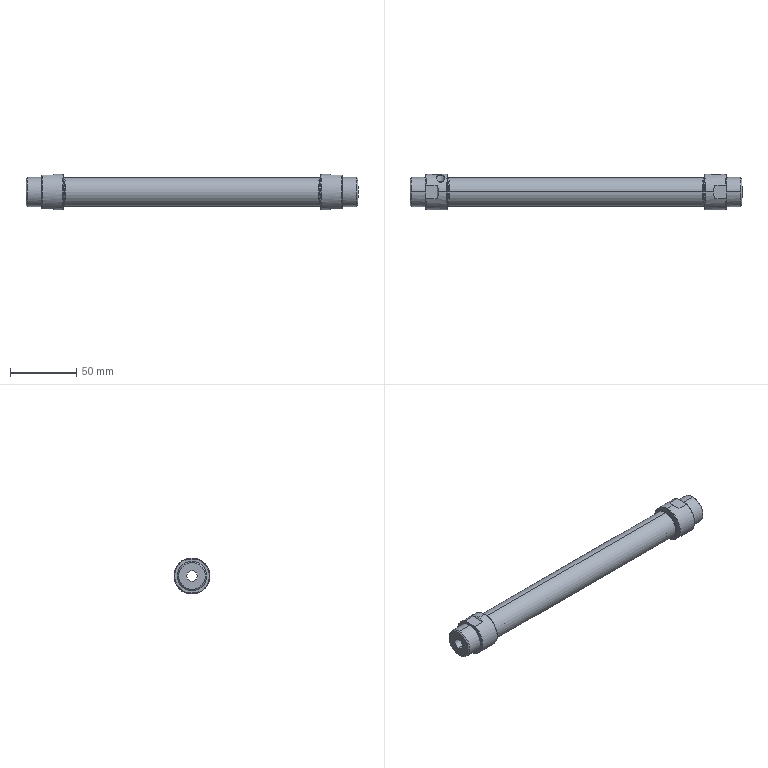Part | STEP file | _20MACJ150Body | 1 solid | 78 faces | box 250 x 27 x 27 mm | volume 37841 mm3 | cylinder 26 | plane 20 | spline 16 | cone 16 | commonest cylinder face diameters 6.5 x6 8 x4 8.566 x4 22 x4 27 x4 20 x2